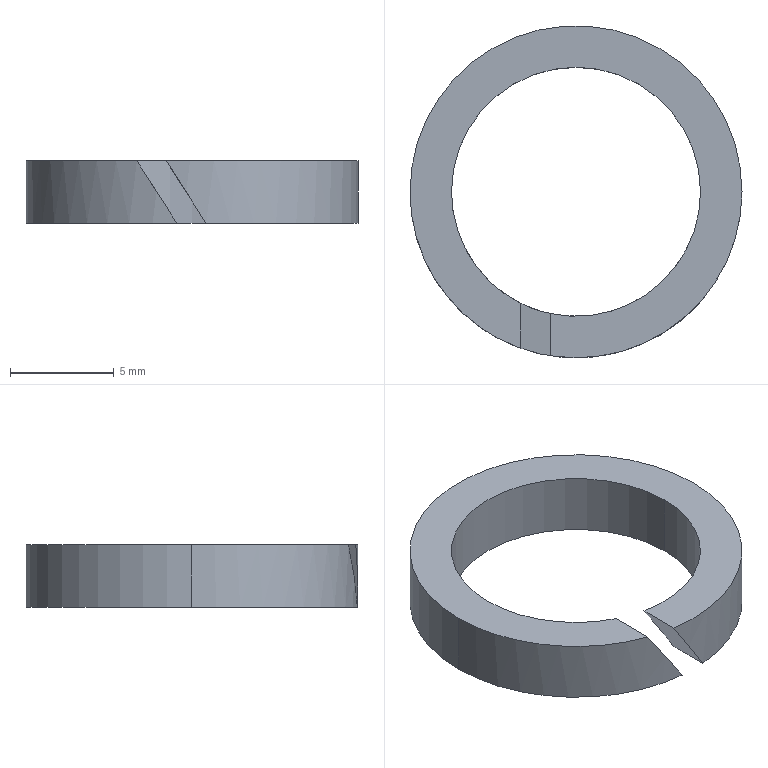Part | SolidWorks | features ICE 1, Revolution 1 | 1 solid | 10 faces | box 16 x 16 x 3 mm | volume 255.282 mm3 | cylinder 6 | plane 4 | commonest cylinder face diameters 12 x3 16 x3
STEP:
#1=CARTESIAN_POINT('',(8.,0.,-7.065));
#2=VERTEX_POINT('',#1);
#3=CARTESIAN_POINT('',(-8.,0.,-7.065));
#4=VERTEX_POINT('',#3);
#5=CARTESIAN_POINT('',(0.,0.,-7.065));
#6=DIRECTION('',(0.,0.,1.));
#7=DIRECTION('',(1.,0.,0.));
#8=AXIS2_PLACEMENT_3D('',#5,#6,#7);
#9=CIRCLE('',#8,8.);
#10=EDGE_CURVE('',#2,#4,#9,.T.);
#11=ORIENTED_EDGE('',*,*,#10,.T.);
#12=CARTESIAN_POINT('',(-8.,0.,-4.065));
#13=VERTEX_POINT('',#12);
#14=CARTESIAN_POINT('',(-8.,0.,0.));
#15=DIRECTION('',(0.,0.,1.));
#16=VECTOR('',#15,1000.);
#17=LINE('',#14,#16);
#18=EDGE_CURVE('',#4,#13,#17,.T.);
#19=ORIENTED_EDGE('',*,*,#18,.T.);
#20=CARTESIAN_POINT('',(8.,0.,-4.065));
#21=VERTEX_POINT('',#20);
#22=CARTESIAN_POINT('',(0.,0.,-4.065));
#23=DIRECTION('',(0.,0.,1.));
#24=DIRECTION('',(1.,0.,0.));
#25=AXIS2_PLACEMENT_3D('',#22,#23,#24);
#26=CIRCLE('',#25,8.);
#27=EDGE_CURVE('',#21,#13,#26,.T.);
#28=ORIENTED_EDGE('',*,*,#27,.F.);
#29=CARTESIAN_POINT('',(8.,0.,0.));
#30=DIRECTION('',(0.,0.,1.));
#31=VECTOR('',#30,1000.);
#32=LINE('',#29,#31);
#33=EDGE_CURVE('',#2,#21,#32,.T.);
#34=ORIENTED_EDGE('',*,*,#33,.F.);
#35=EDGE_LOOP('',(#11,#19,#28,#34));
#36=FACE_OUTER_BOUND('',#35,.T.);
#37=CARTESIAN_POINT('',(0.,0.,0.));
#38=DIRECTION('',(0.,0.,1.));
#39=DIRECTION('',(1.,0.,0.));
#40=AXIS2_PLACEMENT_3D('',#37,#38,#39);
#41=CYLINDRICAL_SURFACE('',#40,8.);
#42=ADVANCED_FACE('',(#36),#41,.T.);
#43=CARTESIAN_POINT('',(0.6787,-7.971,-7.065));
#44=VERTEX_POINT('',#43);
#45=CARTESIAN_POINT('',(0.,0.,-7.065));
#46=DIRECTION('',(0.,0.,1.));
#47=DIRECTION('',(1.,0.,0.));
#48=AXIS2_PLACEMENT_3D('',#45,#46,#47);
#49=CIRCLE('',#48,8.);
#50=EDGE_CURVE('',#44,#2,#49,.T.);
#51=ORIENTED_EDGE('',*,*,#50,.T.);
#52=ORIENTED_EDGE('',*,*,#33,.T.);
#53=CARTESIAN_POINT('',(-1.241,-7.903,-4.065));
#54=VERTEX_POINT('',#53);
#55=CARTESIAN_POINT('',(0.,0.,-4.065));
#56=DIRECTION('',(0.,0.,1.));
#57=DIRECTION('',(1.,0.,0.));
#58=AXIS2_PLACEMENT_3D('',#55,#56,#57);
#59=CIRCLE('',#58,8.);
#60=EDGE_CURVE('',#54,#21,#59,.T.);
#61=ORIENTED_EDGE('',*,*,#60,.F.);
#62=CARTESIAN_POINT('',(0.6787,-7.971,-7.065));
#63=CARTESIAN_POINT('',(0.03769,-8.026,-6.063));
#64=CARTESIAN_POINT('',(-0.6053,-8.003,-5.058));
#65=CARTESIAN_POINT('',(-1.241,-7.903,-4.065));
#66=(BOUNDED_CURVE()B_SPLINE_CURVE(3,(#62,#63,#64,#65),.UNSPECIFIED.,.F.,.F.)B_SPLINE_CURVE_WITH_KNOTS((4,4),(4.627,4.868),.UNSPECIFIED.)CURVE()GEOMETRIC_REPRESENTATION_ITEM()RATIONAL_B_SPLINE_CURVE((1.,0.9952,0.9952,1.))REPRESENTATION_ITEM(''));
#67=EDGE_CURVE('',#44,#54,#66,.T.);
#68=ORIENTED_EDGE('',*,*,#67,.F.);
#69=EDGE_LOOP('',(#51,#52,#61,#68));
#70=FACE_OUTER_BOUND('',#69,.T.);
#71=CARTESIAN_POINT('',(0.,0.,0.));
#72=DIRECTION('',(0.,0.,1.));
#73=DIRECTION('',(1.,0.,0.));
#74=AXIS2_PLACEMENT_3D('',#71,#72,#73);
#75=CYLINDRICAL_SURFACE('',#74,8.);
#76=ADVANCED_FACE('',(#70),#75,.T.);
#77=CARTESIAN_POINT('',(-6.,0.,-7.065));
#78=VERTEX_POINT('',#77);
#79=CARTESIAN_POINT('',(-0.7341,-5.955,-7.065));
#80=VERTEX_POINT('',#79);
#81=CARTESIAN_POINT('',(0.,0.,-7.065));
#82=DIRECTION('',(0.,0.,1.));
#83=DIRECTION('',(1.,0.,0.));
#84=AXIS2_PLACEMENT_3D('',#81,#82,#83);
#85=CIRCLE('',#84,6.);
#86=EDGE_CURVE('',#78,#80,#85,.T.);
#87=ORIENTED_EDGE('',*,*,#86,.F.);
#88=CARTESIAN_POINT('',(-6.,0.,-4.065));
#89=VERTEX_POINT('',#88);
#90=CARTESIAN_POINT('',(-6.,0.,0.));
#91=DIRECTION('',(0.,0.,1.));
#92=VECTOR('',#91,1000.);
#93=LINE('',#90,#92);
#94=EDGE_CURVE('',#78,#89,#93,.T.);
#95=ORIENTED_EDGE('',*,*,#94,.T.);
#96=CARTESIAN_POINT('',(-2.654,-5.381,-4.065));
#97=VERTEX_POINT('',#96);
#98=CARTESIAN_POINT('',(0.,0.,-4.065));
#99=DIRECTION('',(0.,0.,1.));
#100=DIRECTION('',(1.,0.,0.));
#101=AXIS2_PLACEMENT_3D('',#98,#99,#100);
#102=CIRCLE('',#101,6.);
#103=EDGE_CURVE('',#89,#97,#102,.T.);
#104=ORIENTED_EDGE('',*,*,#103,.T.);
#105=CARTESIAN_POINT('',(-0.7341,-5.955,-7.065));
#106=CARTESIAN_POINT('',(-1.403,-5.872,-6.019));
#107=CARTESIAN_POINT('',(-2.049,-5.679,-5.01));
#108=CARTESIAN_POINT('',(-2.654,-5.381,-4.065));
#109=(BOUNDED_CURVE()B_SPLINE_CURVE(3,(#105,#106,#107,#108),.UNSPECIFIED.,.F.,.F.)B_SPLINE_CURVE_WITH_KNOTS((4,4),(4.835,5.171),.UNSPECIFIED.)CURVE()GEOMETRIC_REPRESENTATION_ITEM()RATIONAL_B_SPLINE_CURVE((1.,0.9906,0.9906,1.))REPRESENTATION_ITEM(''));
#110=EDGE_CURVE('',#80,#97,#109,.T.);
#111=ORIENTED_EDGE('',*,*,#110,.F.);
#112=EDGE_LOOP('',(#87,#95,#104,#111));
#113=FACE_OUTER_BOUND('',#112,.T.);
#114=CARTESIAN_POINT('',(0.,0.,0.));
#115=DIRECTION('',(0.,0.,1.));
#116=DIRECTION('',(1.,0.,0.));
#117=AXIS2_PLACEMENT_3D('',#114,#115,#116);
#118=CYLINDRICAL_SURFACE('',#117,6.);
#119=ADVANCED_FACE('',(#113),#118,.F.);
#120=ORIENTED_EDGE('',*,*,#94,.F.);
#121=CARTESIAN_POINT('',(6.,0.,-7.065));
#122=VERTEX_POINT('',#121);
#123=CARTESIAN_POINT('',(0.,0.,-7.065));
#124=DIRECTION('',(0.,0.,1.));
#125=DIRECTION('',(1.,0.,0.));
#126=AXIS2_PLACEMENT_3D('',#123,#124,#125);
#127=CIRCLE('',#126,6.);
#128=EDGE_CURVE('',#122,#78,#127,.T.);
#129=ORIENTED_EDGE('',*,*,#128,.F.);
#130=CARTESIAN_POINT('',(6.,0.,-4.065));
#131=VERTEX_POINT('',#130);
#132=CARTESIAN_POINT('',(6.,0.,0.));
#133=DIRECTION('',(0.,0.,1.));
#134=VECTOR('',#133,1000.);
#135=LINE('',#132,#134);
#136=EDGE_CURVE('',#122,#131,#135,.T.);
#137=ORIENTED_EDGE('',*,*,#136,.T.);
#138=CARTESIAN_POINT('',(0.,0.,-4.065));
#139=DIRECTION('',(0.,0.,1.));
#140=DIRECTION('',(1.,0.,0.));
#141=AXIS2_PLACEMENT_3D('',#138,#139,#140);
#142=CIRCLE('',#141,6.);
#143=EDGE_CURVE('',#131,#89,#142,.T.);
#144=ORIENTED_EDGE('',*,*,#143,.T.);
#145=EDGE_LOOP('',(#120,#129,#137,#144));
#146=FACE_OUTER_BOUND('',#145,.T.);
#147=CARTESIAN_POINT('',(0.,0.,0.));
#148=DIRECTION('',(0.,0.,1.));
#149=DIRECTION('',(1.,0.,0.));
#150=AXIS2_PLACEMENT_3D('',#147,#148,#149);
#151=CYLINDRICAL_SURFACE('',#150,6.);
#152=ADVANCED_FACE('',(#146),#151,.F.);
#153=ORIENTED_EDGE('',*,*,#136,.F.);
#154=CARTESIAN_POINT('',(0.6787,-5.961,-7.065));
#155=VERTEX_POINT('',#154);
#156=CARTESIAN_POINT('',(0.,0.,-7.065));
#157=DIRECTION('',(0.,0.,1.));
#158=DIRECTION('',(1.,0.,0.));
#159=AXIS2_PLACEMENT_3D('',#156,#157,#158);
#160=CIRCLE('',#159,6.);
#161=EDGE_CURVE('',#155,#122,#160,.T.);
#162=ORIENTED_EDGE('',*,*,#161,.F.);
#163=CARTESIAN_POINT('',(-1.241,-5.87,-4.065));
#164=VERTEX_POINT('',#163);
#165=CARTESIAN_POINT('',(-1.241,-5.87,-4.065));
#166=CARTESIAN_POINT('',(-0.6087,-6.004,-5.053));
#167=CARTESIAN_POINT('',(0.03674,-6.035,-6.061));
#168=CARTESIAN_POINT('',(0.6787,-5.961,-7.065));
#169=(BOUNDED_CURVE()B_SPLINE_CURVE(3,(#165,#166,#167,#168),.UNSPECIFIED.,.F.,.F.)B_SPLINE_CURVE_WITH_KNOTS((4,4),(1.362,1.684),.UNSPECIFIED.)CURVE()GEOMETRIC_REPRESENTATION_ITEM()RATIONAL_B_SPLINE_CURVE((1.,0.9914,0.9914,1.))REPRESENTATION_ITEM(''));
#170=EDGE_CURVE('',#164,#155,#169,.T.);
#171=ORIENTED_EDGE('',*,*,#170,.F.);
#172=CARTESIAN_POINT('',(0.,0.,-4.065));
#173=DIRECTION('',(0.,0.,1.));
#174=DIRECTION('',(1.,0.,0.));
#175=AXIS2_PLACEMENT_3D('',#172,#173,#174);
#176=CIRCLE('',#175,6.);
#177=EDGE_CURVE('',#164,#131,#176,.T.);
#178=ORIENTED_EDGE('',*,*,#177,.T.);
#179=EDGE_LOOP('',(#153,#162,#171,#178));
#180=FACE_OUTER_BOUND('',#179,.T.);
#181=CARTESIAN_POINT('',(0.,0.,0.));
#182=DIRECTION('',(0.,0.,1.));
#183=DIRECTION('',(1.,0.,0.));
#184=AXIS2_PLACEMENT_3D('',#181,#182,#183);
#185=CYLINDRICAL_SURFACE('',#184,6.);
#186=ADVANCED_FACE('',(#180),#185,.F.);
#187=CARTESIAN_POINT('',(-0.7341,-7.966,-7.065));
#188=VERTEX_POINT('',#187);
#189=CARTESIAN_POINT('',(-0.7341,0.,-7.065));
#190=DIRECTION('',(0.,1.,0.));
#191=VECTOR('',#190,1000.);
#192=LINE('',#189,#191);
#193=EDGE_CURVE('',#188,#80,#192,.T.);
#194=ORIENTED_EDGE('',*,*,#193,.F.);
#195=CARTESIAN_POINT('',(0.,0.,-7.065));
#196=DIRECTION('',(0.,0.,1.));
#197=DIRECTION('',(1.,0.,0.));
#198=AXIS2_PLACEMENT_3D('',#195,#196,#197);
#199=CIRCLE('',#198,8.);
#200=EDGE_CURVE('',#4,#188,#199,.T.);
#201=ORIENTED_EDGE('',*,*,#200,.F.);
#202=ORIENTED_EDGE('',*,*,#10,.F.);
#203=ORIENTED_EDGE('',*,*,#50,.F.);
#204=CARTESIAN_POINT('',(0.6787,0.,-7.065));
#205=DIRECTION('',(0.,-1.,0.));
#206=VECTOR('',#205,1000.);
#207=LINE('',#204,#206);
#208=EDGE_CURVE('',#155,#44,#207,.T.);
#209=ORIENTED_EDGE('',*,*,#208,.F.);
#210=ORIENTED_EDGE('',*,*,#161,.T.);
#211=ORIENTED_EDGE('',*,*,#128,.T.);
#212=ORIENTED_EDGE('',*,*,#86,.T.);
#213=EDGE_LOOP('',(#194,#201,#202,#203,#209,#210,#211,#212));
#214=FACE_OUTER_BOUND('',#213,.T.);
#215=CARTESIAN_POINT('',(6.,0.,-7.065));
#216=DIRECTION('',(0.,0.,-1.));
#217=DIRECTION('',(-1.,0.,0.));
#218=AXIS2_PLACEMENT_3D('',#215,#216,#217);
#219=PLANE('',#218);
#220=ADVANCED_FACE('',(#214),#219,.T.);
#221=ORIENTED_EDGE('',*,*,#18,.F.);
#222=ORIENTED_EDGE('',*,*,#200,.T.);
#223=CARTESIAN_POINT('',(-2.654,-7.547,-4.065));
#224=VERTEX_POINT('',#223);
#225=CARTESIAN_POINT('',(-2.654,-7.547,-4.065));
#226=CARTESIAN_POINT('',(-2.033,-7.765,-5.035));
#227=CARTESIAN_POINT('',(-1.39,-7.906,-6.04));
#228=CARTESIAN_POINT('',(-0.7341,-7.966,-7.065));
#229=(BOUNDED_CURVE()B_SPLINE_CURVE(3,(#225,#226,#227,#228),.UNSPECIFIED.,.F.,.T.)B_SPLINE_CURVE_WITH_KNOTS((4,4),(1.233,1.479),.UNSPECIFIED.)CURVE()GEOMETRIC_REPRESENTATION_ITEM()RATIONAL_B_SPLINE_CURVE((1.,0.995,0.995,1.))REPRESENTATION_ITEM(''));
#230=EDGE_CURVE('',#224,#188,#229,.T.);
#231=ORIENTED_EDGE('',*,*,#230,.F.);
#232=CARTESIAN_POINT('',(0.,0.,-4.065));
#233=DIRECTION('',(0.,0.,1.));
#234=DIRECTION('',(1.,0.,0.));
#235=AXIS2_PLACEMENT_3D('',#232,#233,#234);
#236=CIRCLE('',#235,8.);
#237=EDGE_CURVE('',#13,#224,#236,.T.);
#238=ORIENTED_EDGE('',*,*,#237,.F.);
#239=EDGE_LOOP('',(#221,#222,#231,#238));
#240=FACE_OUTER_BOUND('',#239,.T.);
#241=CARTESIAN_POINT('',(0.,0.,0.));
#242=DIRECTION('',(0.,0.,1.));
#243=DIRECTION('',(1.,0.,0.));
#244=AXIS2_PLACEMENT_3D('',#241,#242,#243);
#245=CYLINDRICAL_SURFACE('',#244,8.);
#246=ADVANCED_FACE('',(#240),#245,.T.);
#247=CARTESIAN_POINT('',(-2.654,0.,-4.065));
#248=DIRECTION('',(0.,-1.,0.));
#249=VECTOR('',#248,1000.);
#250=LINE('',#247,#249);
#251=EDGE_CURVE('',#97,#224,#250,.T.);
#252=ORIENTED_EDGE('',*,*,#251,.F.);
#253=ORIENTED_EDGE('',*,*,#103,.F.);
#254=ORIENTED_EDGE('',*,*,#143,.F.);
#255=ORIENTED_EDGE('',*,*,#177,.F.);
#256=CARTESIAN_POINT('',(-1.241,0.,-4.065));
#257=DIRECTION('',(0.,1.,0.));
#258=VECTOR('',#257,1000.);
#259=LINE('',#256,#258);
#260=EDGE_CURVE('',#54,#164,#259,.T.);
#261=ORIENTED_EDGE('',*,*,#260,.F.);
#262=ORIENTED_EDGE('',*,*,#60,.T.);
#263=ORIENTED_EDGE('',*,*,#27,.T.);
#264=ORIENTED_EDGE('',*,*,#237,.T.);
#265=EDGE_LOOP('',(#252,#253,#254,#255,#261,#262,#263,#264));
#266=FACE_OUTER_BOUND('',#265,.T.);
#267=CARTESIAN_POINT('',(6.,0.,-4.065));
#268=DIRECTION('',(0.,0.,1.));
#269=DIRECTION('',(1.,0.,0.));
#270=AXIS2_PLACEMENT_3D('',#267,#268,#269);
#271=PLANE('',#270);
#272=ADVANCED_FACE('',(#266),#271,.T.);
#273=ORIENTED_EDGE('',*,*,#170,.T.);
#274=ORIENTED_EDGE('',*,*,#208,.T.);
#275=ORIENTED_EDGE('',*,*,#67,.T.);
#276=ORIENTED_EDGE('',*,*,#260,.T.);
#277=EDGE_LOOP('',(#273,#274,#275,#276));
#278=FACE_OUTER_BOUND('',#277,.T.);
#279=CARTESIAN_POINT('',(3.382,-23.,-11.29));
#280=DIRECTION('',(0.8423,0.,0.539));
#281=DIRECTION('',(0.539,0.,-0.8423));
#282=AXIS2_PLACEMENT_3D('',#279,#280,#281);
#283=PLANE('',#282);
#284=ADVANCED_FACE('',(#278),#283,.F.);
#285=ORIENTED_EDGE('',*,*,#110,.T.);
#286=ORIENTED_EDGE('',*,*,#251,.T.);
#287=ORIENTED_EDGE('',*,*,#230,.T.);
#288=ORIENTED_EDGE('',*,*,#193,.T.);
#289=EDGE_LOOP('',(#285,#286,#287,#288));
#290=FACE_OUTER_BOUND('',#289,.T.);
#291=CARTESIAN_POINT('',(-3.276,-23.,-3.092));
#292=DIRECTION('',(-0.8423,0.,-0.539));
#293=DIRECTION('',(-0.539,0.,0.8423));
#294=AXIS2_PLACEMENT_3D('',#291,#292,#293);
#295=PLANE('',#294);
#296=ADVANCED_FACE('',(#290),#295,.F.);
#297=CLOSED_SHELL('',(#42,#76,#119,#152,#186,#220,#246,#272,#284,#296));
#298=MANIFOLD_SOLID_BREP('',#297);
#299=CARTESIAN_POINT('',(0.,0.,0.));
#300=DIRECTION('',(0.,0.,1.));
#301=DIRECTION('',(1.,0.,0.));
#302=AXIS2_PLACEMENT_3D('',#299,#300,#301);
#303=(LENGTH_UNIT()NAMED_UNIT(*)SI_UNIT(.MILLI.,.METRE.));
#304=UNCERTAINTY_MEASURE_WITH_UNIT(LENGTH_MEASURE(0.00001),#303,'','');
#305=(NAMED_UNIT(*)PLANE_ANGLE_UNIT()SI_UNIT($,.RADIAN.));
#306=(NAMED_UNIT(*)SI_UNIT($,.STERADIAN.)SOLID_ANGLE_UNIT());
#307=(GEOMETRIC_REPRESENTATION_CONTEXT(3)GLOBAL_UNCERTAINTY_ASSIGNED_CONTEXT((#304))GLOBAL_UNIT_ASSIGNED_CONTEXT((#303,#305,#306))REPRESENTATION_CONTEXT('',''));
#308=ADVANCED_BREP_SHAPE_REPRESENTATION('',(#298,#302),#307);